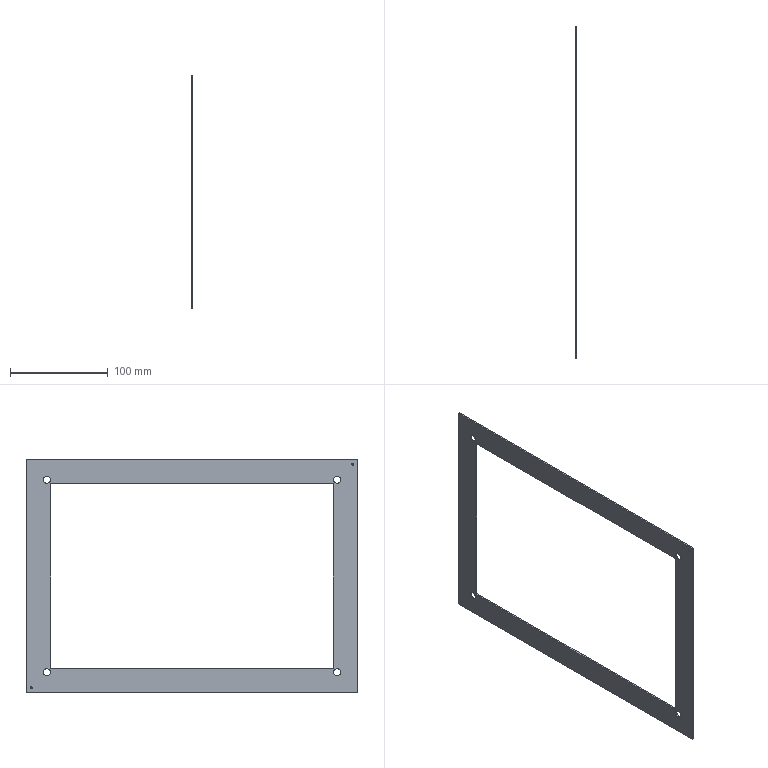Part | SolidWorks | features Extrusion 1 | 1 solid | 22 faces | box 1.5 x 338.6 x 238.5 mm | volume 39286 mm3 | cylinder 12 | plane 10 | commonest cylinder face diameters 7.1 x8 2 x4
STEP:
#1=CARTESIAN_POINT('',(2614.43,1359.3,292.695));
#2=VERTEX_POINT('',#1);
#3=CARTESIAN_POINT('',(2614.43,1359.3,285.595));
#4=VERTEX_POINT('',#3);
#5=CARTESIAN_POINT('',(2614.43,1359.3,289.145));
#6=DIRECTION('',(1.,0.,0.));
#7=DIRECTION('',(0.,0.,1.));
#8=AXIS2_PLACEMENT_3D('',#5,#6,#7);
#9=CIRCLE('',#8,3.55);
#10=EDGE_CURVE('',#2,#4,#9,.T.);
#11=ORIENTED_EDGE('',*,*,#10,.F.);
#12=CARTESIAN_POINT('',(2615.93,1359.3,292.695));
#13=VERTEX_POINT('',#12);
#14=CARTESIAN_POINT('',(2614.43,1359.3,292.695));
#15=DIRECTION('',(1.,0.,0.));
#16=VECTOR('',#15,1000.);
#17=LINE('',#14,#16);
#18=EDGE_CURVE('',#2,#13,#17,.T.);
#19=ORIENTED_EDGE('',*,*,#18,.T.);
#20=CARTESIAN_POINT('',(2615.93,1359.3,285.595));
#21=VERTEX_POINT('',#20);
#22=CARTESIAN_POINT('',(2615.93,1359.3,289.145));
#23=DIRECTION('',(1.,0.,0.));
#24=DIRECTION('',(0.,0.,1.));
#25=AXIS2_PLACEMENT_3D('',#22,#23,#24);
#26=CIRCLE('',#25,3.55);
#27=EDGE_CURVE('',#13,#21,#26,.T.);
#28=ORIENTED_EDGE('',*,*,#27,.T.);
#29=CARTESIAN_POINT('',(2614.43,1359.3,285.595));
#30=DIRECTION('',(1.,0.,0.));
#31=VECTOR('',#30,1000.);
#32=LINE('',#29,#31);
#33=EDGE_CURVE('',#4,#21,#32,.T.);
#34=ORIENTED_EDGE('',*,*,#33,.F.);
#35=EDGE_LOOP('',(#11,#19,#28,#34));
#36=FACE_OUTER_BOUND('',#35,.T.);
#37=CARTESIAN_POINT('',(2614.43,1359.3,289.145));
#38=DIRECTION('',(1.,0.,0.));
#39=DIRECTION('',(0.,0.,-1.));
#40=AXIS2_PLACEMENT_3D('',#37,#38,#39);
#41=CYLINDRICAL_SURFACE('',#40,3.55);
#42=ADVANCED_FACE('',(#36),#41,.F.);
#43=CARTESIAN_POINT('',(2614.43,1062.7,96.195));
#44=VERTEX_POINT('',#43);
#45=CARTESIAN_POINT('',(2614.43,1062.7,89.095));
#46=VERTEX_POINT('',#45);
#47=CARTESIAN_POINT('',(2614.43,1062.7,92.645));
#48=DIRECTION('',(1.,0.,0.));
#49=DIRECTION('',(0.,0.,1.));
#50=AXIS2_PLACEMENT_3D('',#47,#48,#49);
#51=CIRCLE('',#50,3.55);
#52=EDGE_CURVE('',#44,#46,#51,.T.);
#53=ORIENTED_EDGE('',*,*,#52,.F.);
#54=CARTESIAN_POINT('',(2615.93,1062.7,96.195));
#55=VERTEX_POINT('',#54);
#56=CARTESIAN_POINT('',(2614.43,1062.7,96.195));
#57=DIRECTION('',(1.,0.,0.));
#58=VECTOR('',#57,1000.);
#59=LINE('',#56,#58);
#60=EDGE_CURVE('',#44,#55,#59,.T.);
#61=ORIENTED_EDGE('',*,*,#60,.T.);
#62=CARTESIAN_POINT('',(2615.93,1062.7,89.095));
#63=VERTEX_POINT('',#62);
#64=CARTESIAN_POINT('',(2615.93,1062.7,92.645));
#65=DIRECTION('',(1.,0.,0.));
#66=DIRECTION('',(0.,0.,1.));
#67=AXIS2_PLACEMENT_3D('',#64,#65,#66);
#68=CIRCLE('',#67,3.55);
#69=EDGE_CURVE('',#55,#63,#68,.T.);
#70=ORIENTED_EDGE('',*,*,#69,.T.);
#71=CARTESIAN_POINT('',(2614.43,1062.7,89.095));
#72=DIRECTION('',(1.,0.,0.));
#73=VECTOR('',#72,1000.);
#74=LINE('',#71,#73);
#75=EDGE_CURVE('',#46,#63,#74,.T.);
#76=ORIENTED_EDGE('',*,*,#75,.F.);
#77=EDGE_LOOP('',(#53,#61,#70,#76));
#78=FACE_OUTER_BOUND('',#77,.T.);
#79=CARTESIAN_POINT('',(2614.43,1062.7,92.645));
#80=DIRECTION('',(1.,0.,0.));
#81=DIRECTION('',(0.,0.,-1.));
#82=AXIS2_PLACEMENT_3D('',#79,#80,#81);
#83=CYLINDRICAL_SURFACE('',#82,3.55);
#84=ADVANCED_FACE('',(#78),#83,.F.);
#85=CARTESIAN_POINT('',(2614.43,1359.3,96.195));
#86=VERTEX_POINT('',#85);
#87=CARTESIAN_POINT('',(2614.43,1359.3,89.095));
#88=VERTEX_POINT('',#87);
#89=CARTESIAN_POINT('',(2614.43,1359.3,92.645));
#90=DIRECTION('',(1.,0.,0.));
#91=DIRECTION('',(0.,0.,1.));
#92=AXIS2_PLACEMENT_3D('',#89,#90,#91);
#93=CIRCLE('',#92,3.55);
#94=EDGE_CURVE('',#86,#88,#93,.T.);
#95=ORIENTED_EDGE('',*,*,#94,.F.);
#96=CARTESIAN_POINT('',(2615.93,1359.3,96.195));
#97=VERTEX_POINT('',#96);
#98=CARTESIAN_POINT('',(2614.43,1359.3,96.195));
#99=DIRECTION('',(1.,0.,0.));
#100=VECTOR('',#99,1000.);
#101=LINE('',#98,#100);
#102=EDGE_CURVE('',#86,#97,#101,.T.);
#103=ORIENTED_EDGE('',*,*,#102,.T.);
#104=CARTESIAN_POINT('',(2615.93,1359.3,89.095));
#105=VERTEX_POINT('',#104);
#106=CARTESIAN_POINT('',(2615.93,1359.3,92.645));
#107=DIRECTION('',(1.,0.,0.));
#108=DIRECTION('',(0.,0.,1.));
#109=AXIS2_PLACEMENT_3D('',#106,#107,#108);
#110=CIRCLE('',#109,3.55);
#111=EDGE_CURVE('',#97,#105,#110,.T.);
#112=ORIENTED_EDGE('',*,*,#111,.T.);
#113=CARTESIAN_POINT('',(2614.43,1359.3,89.095));
#114=DIRECTION('',(1.,0.,0.));
#115=VECTOR('',#114,1000.);
#116=LINE('',#113,#115);
#117=EDGE_CURVE('',#88,#105,#116,.T.);
#118=ORIENTED_EDGE('',*,*,#117,.F.);
#119=EDGE_LOOP('',(#95,#103,#112,#118));
#120=FACE_OUTER_BOUND('',#119,.T.);
#121=CARTESIAN_POINT('',(2614.43,1359.3,92.645));
#122=DIRECTION('',(1.,0.,0.));
#123=DIRECTION('',(0.,0.,-1.));
#124=AXIS2_PLACEMENT_3D('',#121,#122,#123);
#125=CYLINDRICAL_SURFACE('',#124,3.55);
#126=ADVANCED_FACE('',(#120),#125,.F.);
#127=CARTESIAN_POINT('',(2614.43,1062.7,292.695));
#128=VERTEX_POINT('',#127);
#129=CARTESIAN_POINT('',(2614.43,1062.7,285.595));
#130=VERTEX_POINT('',#129);
#131=CARTESIAN_POINT('',(2614.43,1062.7,289.145));
#132=DIRECTION('',(1.,0.,0.));
#133=DIRECTION('',(0.,0.,1.));
#134=AXIS2_PLACEMENT_3D('',#131,#132,#133);
#135=CIRCLE('',#134,3.55);
#136=EDGE_CURVE('',#128,#130,#135,.T.);
#137=ORIENTED_EDGE('',*,*,#136,.F.);
#138=CARTESIAN_POINT('',(2615.93,1062.7,292.695));
#139=VERTEX_POINT('',#138);
#140=CARTESIAN_POINT('',(2614.43,1062.7,292.695));
#141=DIRECTION('',(1.,0.,0.));
#142=VECTOR('',#141,1000.);
#143=LINE('',#140,#142);
#144=EDGE_CURVE('',#128,#139,#143,.T.);
#145=ORIENTED_EDGE('',*,*,#144,.T.);
#146=CARTESIAN_POINT('',(2615.93,1062.7,285.595));
#147=VERTEX_POINT('',#146);
#148=CARTESIAN_POINT('',(2615.93,1062.7,289.145));
#149=DIRECTION('',(1.,0.,0.));
#150=DIRECTION('',(0.,0.,1.));
#151=AXIS2_PLACEMENT_3D('',#148,#149,#150);
#152=CIRCLE('',#151,3.55);
#153=EDGE_CURVE('',#139,#147,#152,.T.);
#154=ORIENTED_EDGE('',*,*,#153,.T.);
#155=CARTESIAN_POINT('',(2614.43,1062.7,285.595));
#156=DIRECTION('',(1.,0.,0.));
#157=VECTOR('',#156,1000.);
#158=LINE('',#155,#157);
#159=EDGE_CURVE('',#130,#147,#158,.T.);
#160=ORIENTED_EDGE('',*,*,#159,.F.);
#161=EDGE_LOOP('',(#137,#145,#154,#160));
#162=FACE_OUTER_BOUND('',#161,.T.);
#163=CARTESIAN_POINT('',(2614.43,1062.7,289.145));
#164=DIRECTION('',(1.,0.,0.));
#165=DIRECTION('',(0.,0.,-1.));
#166=AXIS2_PLACEMENT_3D('',#163,#164,#165);
#167=CYLINDRICAL_SURFACE('',#166,3.55);
#168=ADVANCED_FACE('',(#162),#167,.F.);
#169=CARTESIAN_POINT('',(2614.43,1375.3,77.645));
#170=VERTEX_POINT('',#169);
#171=CARTESIAN_POINT('',(2614.43,1375.3,75.645));
#172=VERTEX_POINT('',#171);
#173=CARTESIAN_POINT('',(2614.43,1375.3,76.645));
#174=DIRECTION('',(1.,0.,0.));
#175=DIRECTION('',(0.,0.,1.));
#176=AXIS2_PLACEMENT_3D('',#173,#174,#175);
#177=CIRCLE('',#176,1.);
#178=EDGE_CURVE('',#170,#172,#177,.T.);
#179=ORIENTED_EDGE('',*,*,#178,.F.);
#180=CARTESIAN_POINT('',(2615.93,1375.3,77.645));
#181=VERTEX_POINT('',#180);
#182=CARTESIAN_POINT('',(2614.43,1375.3,77.645));
#183=DIRECTION('',(1.,0.,0.));
#184=VECTOR('',#183,1000.);
#185=LINE('',#182,#184);
#186=EDGE_CURVE('',#170,#181,#185,.T.);
#187=ORIENTED_EDGE('',*,*,#186,.T.);
#188=CARTESIAN_POINT('',(2615.93,1375.3,75.645));
#189=VERTEX_POINT('',#188);
#190=CARTESIAN_POINT('',(2615.93,1375.3,76.645));
#191=DIRECTION('',(1.,0.,0.));
#192=DIRECTION('',(0.,0.,1.));
#193=AXIS2_PLACEMENT_3D('',#190,#191,#192);
#194=CIRCLE('',#193,1.);
#195=EDGE_CURVE('',#181,#189,#194,.T.);
#196=ORIENTED_EDGE('',*,*,#195,.T.);
#197=CARTESIAN_POINT('',(2614.43,1375.3,75.645));
#198=DIRECTION('',(1.,0.,0.));
#199=VECTOR('',#198,1000.);
#200=LINE('',#197,#199);
#201=EDGE_CURVE('',#172,#189,#200,.T.);
#202=ORIENTED_EDGE('',*,*,#201,.F.);
#203=EDGE_LOOP('',(#179,#187,#196,#202));
#204=FACE_OUTER_BOUND('',#203,.T.);
#205=CARTESIAN_POINT('',(2614.43,1375.3,76.645));
#206=DIRECTION('',(1.,0.,0.));
#207=DIRECTION('',(0.,0.,-1.));
#208=AXIS2_PLACEMENT_3D('',#205,#206,#207);
#209=CYLINDRICAL_SURFACE('',#208,1.);
#210=ADVANCED_FACE('',(#204),#209,.F.);
#211=CARTESIAN_POINT('',(2614.43,1046.7,306.145));
#212=VERTEX_POINT('',#211);
#213=CARTESIAN_POINT('',(2614.43,1046.7,304.145));
#214=VERTEX_POINT('',#213);
#215=CARTESIAN_POINT('',(2614.43,1046.7,305.145));
#216=DIRECTION('',(1.,0.,0.));
#217=DIRECTION('',(0.,0.,1.));
#218=AXIS2_PLACEMENT_3D('',#215,#216,#217);
#219=CIRCLE('',#218,1.);
#220=EDGE_CURVE('',#212,#214,#219,.T.);
#221=ORIENTED_EDGE('',*,*,#220,.F.);
#222=CARTESIAN_POINT('',(2615.93,1046.7,306.145));
#223=VERTEX_POINT('',#222);
#224=CARTESIAN_POINT('',(2614.43,1046.7,306.145));
#225=DIRECTION('',(1.,0.,0.));
#226=VECTOR('',#225,1000.);
#227=LINE('',#224,#226);
#228=EDGE_CURVE('',#212,#223,#227,.T.);
#229=ORIENTED_EDGE('',*,*,#228,.T.);
#230=CARTESIAN_POINT('',(2615.93,1046.7,304.145));
#231=VERTEX_POINT('',#230);
#232=CARTESIAN_POINT('',(2615.93,1046.7,305.145));
#233=DIRECTION('',(1.,0.,0.));
#234=DIRECTION('',(0.,0.,1.));
#235=AXIS2_PLACEMENT_3D('',#232,#233,#234);
#236=CIRCLE('',#235,1.);
#237=EDGE_CURVE('',#223,#231,#236,.T.);
#238=ORIENTED_EDGE('',*,*,#237,.T.);
#239=CARTESIAN_POINT('',(2614.43,1046.7,304.145));
#240=DIRECTION('',(1.,0.,0.));
#241=VECTOR('',#240,1000.);
#242=LINE('',#239,#241);
#243=EDGE_CURVE('',#214,#231,#242,.T.);
#244=ORIENTED_EDGE('',*,*,#243,.F.);
#245=EDGE_LOOP('',(#221,#229,#238,#244));
#246=FACE_OUTER_BOUND('',#245,.T.);
#247=CARTESIAN_POINT('',(2614.43,1046.7,305.145));
#248=DIRECTION('',(1.,0.,0.));
#249=DIRECTION('',(0.,0.,-1.));
#250=AXIS2_PLACEMENT_3D('',#247,#248,#249);
#251=CYLINDRICAL_SURFACE('',#250,1.);
#252=ADVANCED_FACE('',(#246),#251,.F.);
#253=CARTESIAN_POINT('',(2615.93,1380.3,310.145));
#254=VERTEX_POINT('',#253);
#255=CARTESIAN_POINT('',(2615.93,1041.7,310.145));
#256=VERTEX_POINT('',#255);
#257=CARTESIAN_POINT('',(2615.93,1380.3,310.145));
#258=DIRECTION('',(0.,-1.,0.));
#259=VECTOR('',#258,1000.);
#260=LINE('',#257,#259);
#261=EDGE_CURVE('',#254,#256,#260,.T.);
#262=ORIENTED_EDGE('',*,*,#261,.F.);
#263=CARTESIAN_POINT('',(2614.43,1380.3,310.145));
#264=VERTEX_POINT('',#263);
#265=CARTESIAN_POINT('',(2614.43,1380.3,310.145));
#266=DIRECTION('',(1.,0.,0.));
#267=VECTOR('',#266,1000.);
#268=LINE('',#265,#267);
#269=EDGE_CURVE('',#264,#254,#268,.T.);
#270=ORIENTED_EDGE('',*,*,#269,.F.);
#271=CARTESIAN_POINT('',(2614.43,1041.7,310.145));
#272=VERTEX_POINT('',#271);
#273=CARTESIAN_POINT('',(2614.43,1380.3,310.145));
#274=DIRECTION('',(0.,-1.,0.));
#275=VECTOR('',#274,1000.);
#276=LINE('',#273,#275);
#277=EDGE_CURVE('',#264,#272,#276,.T.);
#278=ORIENTED_EDGE('',*,*,#277,.T.);
#279=CARTESIAN_POINT('',(2614.43,1041.7,310.145));
#280=DIRECTION('',(1.,0.,0.));
#281=VECTOR('',#280,1000.);
#282=LINE('',#279,#281);
#283=EDGE_CURVE('',#272,#256,#282,.T.);
#284=ORIENTED_EDGE('',*,*,#283,.T.);
#285=EDGE_LOOP('',(#262,#270,#278,#284));
#286=FACE_OUTER_BOUND('',#285,.T.);
#287=CARTESIAN_POINT('',(2614.43,1380.3,310.145));
#288=DIRECTION('',(0.,0.,1.));
#289=DIRECTION('',(0.,-1.,0.));
#290=AXIS2_PLACEMENT_3D('',#287,#288,#289);
#291=PLANE('',#290);
#292=ADVANCED_FACE('',(#286),#291,.T.);
#293=CARTESIAN_POINT('',(2615.93,1380.3,71.645));
#294=VERTEX_POINT('',#293);
#295=CARTESIAN_POINT('',(2615.93,1380.3,71.645));
#296=DIRECTION('',(0.,0.,1.));
#297=VECTOR('',#296,1000.);
#298=LINE('',#295,#297);
#299=EDGE_CURVE('',#294,#254,#298,.T.);
#300=ORIENTED_EDGE('',*,*,#299,.F.);
#301=CARTESIAN_POINT('',(2614.43,1380.3,71.645));
#302=VERTEX_POINT('',#301);
#303=CARTESIAN_POINT('',(2614.43,1380.3,71.645));
#304=DIRECTION('',(1.,0.,0.));
#305=VECTOR('',#304,1000.);
#306=LINE('',#303,#305);
#307=EDGE_CURVE('',#302,#294,#306,.T.);
#308=ORIENTED_EDGE('',*,*,#307,.F.);
#309=CARTESIAN_POINT('',(2614.43,1380.3,71.645));
#310=DIRECTION('',(0.,0.,1.));
#311=VECTOR('',#310,1000.);
#312=LINE('',#309,#311);
#313=EDGE_CURVE('',#302,#264,#312,.T.);
#314=ORIENTED_EDGE('',*,*,#313,.T.);
#315=ORIENTED_EDGE('',*,*,#269,.T.);
#316=EDGE_LOOP('',(#300,#308,#314,#315));
#317=FACE_OUTER_BOUND('',#316,.T.);
#318=CARTESIAN_POINT('',(2614.43,1380.3,71.645));
#319=DIRECTION('',(0.,1.,0.));
#320=DIRECTION('',(0.,0.,1.));
#321=AXIS2_PLACEMENT_3D('',#318,#319,#320);
#322=PLANE('',#321);
#323=ADVANCED_FACE('',(#317),#322,.T.);
#324=CARTESIAN_POINT('',(2615.93,1041.7,71.645));
#325=VERTEX_POINT('',#324);
#326=CARTESIAN_POINT('',(2615.93,1041.7,71.645));
#327=DIRECTION('',(0.,1.,0.));
#328=VECTOR('',#327,1000.);
#329=LINE('',#326,#328);
#330=EDGE_CURVE('',#325,#294,#329,.T.);
#331=ORIENTED_EDGE('',*,*,#330,.F.);
#332=CARTESIAN_POINT('',(2614.43,1041.7,71.645));
#333=VERTEX_POINT('',#332);
#334=CARTESIAN_POINT('',(2614.43,1041.7,71.645));
#335=DIRECTION('',(1.,0.,0.));
#336=VECTOR('',#335,1000.);
#337=LINE('',#334,#336);
#338=EDGE_CURVE('',#333,#325,#337,.T.);
#339=ORIENTED_EDGE('',*,*,#338,.F.);
#340=CARTESIAN_POINT('',(2614.43,1041.7,71.645));
#341=DIRECTION('',(0.,1.,0.));
#342=VECTOR('',#341,1000.);
#343=LINE('',#340,#342);
#344=EDGE_CURVE('',#333,#302,#343,.T.);
#345=ORIENTED_EDGE('',*,*,#344,.T.);
#346=ORIENTED_EDGE('',*,*,#307,.T.);
#347=EDGE_LOOP('',(#331,#339,#345,#346));
#348=FACE_OUTER_BOUND('',#347,.T.);
#349=CARTESIAN_POINT('',(2614.43,1041.7,71.645));
#350=DIRECTION('',(0.,0.,-1.));
#351=DIRECTION('',(0.,1.,0.));
#352=AXIS2_PLACEMENT_3D('',#349,#350,#351);
#353=PLANE('',#352);
#354=ADVANCED_FACE('',(#348),#353,.T.);
#355=CARTESIAN_POINT('',(2615.93,1041.7,310.145));
#356=DIRECTION('',(0.,0.,-1.));
#357=VECTOR('',#356,1000.);
#358=LINE('',#355,#357);
#359=EDGE_CURVE('',#256,#325,#358,.T.);
#360=ORIENTED_EDGE('',*,*,#359,.F.);
#361=ORIENTED_EDGE('',*,*,#283,.F.);
#362=CARTESIAN_POINT('',(2614.43,1041.7,310.145));
#363=DIRECTION('',(0.,0.,-1.));
#364=VECTOR('',#363,1000.);
#365=LINE('',#362,#364);
#366=EDGE_CURVE('',#272,#333,#365,.T.);
#367=ORIENTED_EDGE('',*,*,#366,.T.);
#368=ORIENTED_EDGE('',*,*,#338,.T.);
#369=EDGE_LOOP('',(#360,#361,#367,#368));
#370=FACE_OUTER_BOUND('',#369,.T.);
#371=CARTESIAN_POINT('',(2614.43,1041.7,310.145));
#372=DIRECTION('',(0.,-1.,0.));
#373=DIRECTION('',(0.,0.,-1.));
#374=AXIS2_PLACEMENT_3D('',#371,#372,#373);
#375=PLANE('',#374);
#376=ADVANCED_FACE('',(#370),#375,.T.);
#377=CARTESIAN_POINT('',(2614.43,1355.3,285.145));
#378=VERTEX_POINT('',#377);
#379=CARTESIAN_POINT('',(2614.43,1066.7,285.145));
#380=VERTEX_POINT('',#379);
#381=CARTESIAN_POINT('',(2614.43,1066.7,285.145));
#382=DIRECTION('',(0.,-1.,0.));
#383=VECTOR('',#382,1000.);
#384=LINE('',#381,#383);
#385=EDGE_CURVE('',#378,#380,#384,.T.);
#386=ORIENTED_EDGE('',*,*,#385,.T.);
#387=CARTESIAN_POINT('',(2614.43,1066.7,96.645));
#388=VERTEX_POINT('',#387);
#389=CARTESIAN_POINT('',(2614.43,1066.7,96.645));
#390=DIRECTION('',(0.,0.,-1.));
#391=VECTOR('',#390,1000.);
#392=LINE('',#389,#391);
#393=EDGE_CURVE('',#380,#388,#392,.T.);
#394=ORIENTED_EDGE('',*,*,#393,.T.);
#395=CARTESIAN_POINT('',(2614.43,1355.3,96.645));
#396=VERTEX_POINT('',#395);
#397=CARTESIAN_POINT('',(2614.43,1355.3,96.645));
#398=DIRECTION('',(0.,1.,0.));
#399=VECTOR('',#398,1000.);
#400=LINE('',#397,#399);
#401=EDGE_CURVE('',#388,#396,#400,.T.);
#402=ORIENTED_EDGE('',*,*,#401,.T.);
#403=CARTESIAN_POINT('',(2614.43,1355.3,285.145));
#404=DIRECTION('',(0.,0.,1.));
#405=VECTOR('',#404,1000.);
#406=LINE('',#403,#405);
#407=EDGE_CURVE('',#396,#378,#406,.T.);
#408=ORIENTED_EDGE('',*,*,#407,.T.);
#409=EDGE_LOOP('',(#386,#394,#402,#408));
#410=FACE_BOUND('',#409,.T.);
#411=CARTESIAN_POINT('',(2614.43,1359.3,289.145));
#412=DIRECTION('',(1.,0.,0.));
#413=DIRECTION('',(0.,0.,1.));
#414=AXIS2_PLACEMENT_3D('',#411,#412,#413);
#415=CIRCLE('',#414,3.55);
#416=EDGE_CURVE('',#4,#2,#415,.T.);
#417=ORIENTED_EDGE('',*,*,#416,.T.);
#418=ORIENTED_EDGE('',*,*,#10,.T.);
#419=EDGE_LOOP('',(#417,#418));
#420=FACE_BOUND('',#419,.T.);
#421=CARTESIAN_POINT('',(2614.43,1062.7,92.645));
#422=DIRECTION('',(1.,0.,0.));
#423=DIRECTION('',(0.,0.,1.));
#424=AXIS2_PLACEMENT_3D('',#421,#422,#423);
#425=CIRCLE('',#424,3.55);
#426=EDGE_CURVE('',#46,#44,#425,.T.);
#427=ORIENTED_EDGE('',*,*,#426,.T.);
#428=ORIENTED_EDGE('',*,*,#52,.T.);
#429=EDGE_LOOP('',(#427,#428));
#430=FACE_BOUND('',#429,.T.);
#431=CARTESIAN_POINT('',(2614.43,1359.3,92.645));
#432=DIRECTION('',(1.,0.,0.));
#433=DIRECTION('',(0.,0.,1.));
#434=AXIS2_PLACEMENT_3D('',#431,#432,#433);
#435=CIRCLE('',#434,3.55);
#436=EDGE_CURVE('',#88,#86,#435,.T.);
#437=ORIENTED_EDGE('',*,*,#436,.T.);
#438=ORIENTED_EDGE('',*,*,#94,.T.);
#439=EDGE_LOOP('',(#437,#438));
#440=FACE_BOUND('',#439,.T.);
#441=CARTESIAN_POINT('',(2614.43,1062.7,289.145));
#442=DIRECTION('',(1.,0.,0.));
#443=DIRECTION('',(0.,0.,1.));
#444=AXIS2_PLACEMENT_3D('',#441,#442,#443);
#445=CIRCLE('',#444,3.55);
#446=EDGE_CURVE('',#130,#128,#445,.T.);
#447=ORIENTED_EDGE('',*,*,#446,.T.);
#448=ORIENTED_EDGE('',*,*,#136,.T.);
#449=EDGE_LOOP('',(#447,#448));
#450=FACE_BOUND('',#449,.T.);
#451=CARTESIAN_POINT('',(2614.43,1375.3,76.645));
#452=DIRECTION('',(1.,0.,0.));
#453=DIRECTION('',(0.,0.,1.));
#454=AXIS2_PLACEMENT_3D('',#451,#452,#453);
#455=CIRCLE('',#454,1.);
#456=EDGE_CURVE('',#172,#170,#455,.T.);
#457=ORIENTED_EDGE('',*,*,#456,.T.);
#458=ORIENTED_EDGE('',*,*,#178,.T.);
#459=EDGE_LOOP('',(#457,#458));
#460=FACE_BOUND('',#459,.T.);
#461=CARTESIAN_POINT('',(2614.43,1046.7,305.145));
#462=DIRECTION('',(1.,0.,0.));
#463=DIRECTION('',(0.,0.,1.));
#464=AXIS2_PLACEMENT_3D('',#461,#462,#463);
#465=CIRCLE('',#464,1.);
#466=EDGE_CURVE('',#214,#212,#465,.T.);
#467=ORIENTED_EDGE('',*,*,#466,.T.);
#468=ORIENTED_EDGE('',*,*,#220,.T.);
#469=EDGE_LOOP('',(#467,#468));
#470=FACE_BOUND('',#469,.T.);
#471=ORIENTED_EDGE('',*,*,#277,.F.);
#472=ORIENTED_EDGE('',*,*,#313,.F.);
#473=ORIENTED_EDGE('',*,*,#344,.F.);
#474=ORIENTED_EDGE('',*,*,#366,.F.);
#475=EDGE_LOOP('',(#471,#472,#473,#474));
#476=FACE_OUTER_BOUND('',#475,.T.);
#477=CARTESIAN_POINT('',(2614.43,0.,0.));
#478=DIRECTION('',(1.,0.,0.));
#479=DIRECTION('',(0.,0.,-1.));
#480=AXIS2_PLACEMENT_3D('',#477,#478,#479);
#481=PLANE('',#480);
#482=ADVANCED_FACE('',(#410,#420,#430,#440,#450,#460,#470,#476),#481,.F.);
#483=CARTESIAN_POINT('',(2615.93,1066.7,285.145));
#484=VERTEX_POINT('',#483);
#485=CARTESIAN_POINT('',(2615.93,1066.7,96.645));
#486=VERTEX_POINT('',#485);
#487=CARTESIAN_POINT('',(2615.93,1066.7,96.645));
#488=DIRECTION('',(0.,0.,-1.));
#489=VECTOR('',#488,1000.);
#490=LINE('',#487,#489);
#491=EDGE_CURVE('',#484,#486,#490,.T.);
#492=ORIENTED_EDGE('',*,*,#491,.F.);
#493=CARTESIAN_POINT('',(2615.93,1355.3,285.145));
#494=VERTEX_POINT('',#493);
#495=CARTESIAN_POINT('',(2615.93,1066.7,285.145));
#496=DIRECTION('',(0.,-1.,0.));
#497=VECTOR('',#496,1000.);
#498=LINE('',#495,#497);
#499=EDGE_CURVE('',#494,#484,#498,.T.);
#500=ORIENTED_EDGE('',*,*,#499,.F.);
#501=CARTESIAN_POINT('',(2615.93,1355.3,96.645));
#502=VERTEX_POINT('',#501);
#503=CARTESIAN_POINT('',(2615.93,1355.3,285.145));
#504=DIRECTION('',(0.,0.,1.));
#505=VECTOR('',#504,1000.);
#506=LINE('',#503,#505);
#507=EDGE_CURVE('',#502,#494,#506,.T.);
#508=ORIENTED_EDGE('',*,*,#507,.F.);
#509=CARTESIAN_POINT('',(2615.93,1355.3,96.645));
#510=DIRECTION('',(0.,1.,0.));
#511=VECTOR('',#510,1000.);
#512=LINE('',#509,#511);
#513=EDGE_CURVE('',#486,#502,#512,.T.);
#514=ORIENTED_EDGE('',*,*,#513,.F.);
#515=EDGE_LOOP('',(#492,#500,#508,#514));
#516=FACE_BOUND('',#515,.T.);
#517=CARTESIAN_POINT('',(2615.93,1359.3,289.145));
#518=DIRECTION('',(1.,0.,0.));
#519=DIRECTION('',(0.,0.,1.));
#520=AXIS2_PLACEMENT_3D('',#517,#518,#519);
#521=CIRCLE('',#520,3.55);
#522=EDGE_CURVE('',#21,#13,#521,.T.);
#523=ORIENTED_EDGE('',*,*,#522,.F.);
#524=ORIENTED_EDGE('',*,*,#27,.F.);
#525=EDGE_LOOP('',(#523,#524));
#526=FACE_BOUND('',#525,.T.);
#527=CARTESIAN_POINT('',(2615.93,1062.7,92.645));
#528=DIRECTION('',(1.,0.,0.));
#529=DIRECTION('',(0.,0.,1.));
#530=AXIS2_PLACEMENT_3D('',#527,#528,#529);
#531=CIRCLE('',#530,3.55);
#532=EDGE_CURVE('',#63,#55,#531,.T.);
#533=ORIENTED_EDGE('',*,*,#532,.F.);
#534=ORIENTED_EDGE('',*,*,#69,.F.);
#535=EDGE_LOOP('',(#533,#534));
#536=FACE_BOUND('',#535,.T.);
#537=CARTESIAN_POINT('',(2615.93,1359.3,92.645));
#538=DIRECTION('',(1.,0.,0.));
#539=DIRECTION('',(0.,0.,1.));
#540=AXIS2_PLACEMENT_3D('',#537,#538,#539);
#541=CIRCLE('',#540,3.55);
#542=EDGE_CURVE('',#105,#97,#541,.T.);
#543=ORIENTED_EDGE('',*,*,#542,.F.);
#544=ORIENTED_EDGE('',*,*,#111,.F.);
#545=EDGE_LOOP('',(#543,#544));
#546=FACE_BOUND('',#545,.T.);
#547=CARTESIAN_POINT('',(2615.93,1062.7,289.145));
#548=DIRECTION('',(1.,0.,0.));
#549=DIRECTION('',(0.,0.,1.));
#550=AXIS2_PLACEMENT_3D('',#547,#548,#549);
#551=CIRCLE('',#550,3.55);
#552=EDGE_CURVE('',#147,#139,#551,.T.);
#553=ORIENTED_EDGE('',*,*,#552,.F.);
#554=ORIENTED_EDGE('',*,*,#153,.F.);
#555=EDGE_LOOP('',(#553,#554));
#556=FACE_BOUND('',#555,.T.);
#557=CARTESIAN_POINT('',(2615.93,1375.3,76.645));
#558=DIRECTION('',(1.,0.,0.));
#559=DIRECTION('',(0.,0.,1.));
#560=AXIS2_PLACEMENT_3D('',#557,#558,#559);
#561=CIRCLE('',#560,1.);
#562=EDGE_CURVE('',#189,#181,#561,.T.);
#563=ORIENTED_EDGE('',*,*,#562,.F.);
#564=ORIENTED_EDGE('',*,*,#195,.F.);
#565=EDGE_LOOP('',(#563,#564));
#566=FACE_BOUND('',#565,.T.);
#567=CARTESIAN_POINT('',(2615.93,1046.7,305.145));
#568=DIRECTION('',(1.,0.,0.));
#569=DIRECTION('',(0.,0.,1.));
#570=AXIS2_PLACEMENT_3D('',#567,#568,#569);
#571=CIRCLE('',#570,1.);
#572=EDGE_CURVE('',#231,#223,#571,.T.);
#573=ORIENTED_EDGE('',*,*,#572,.F.);
#574=ORIENTED_EDGE('',*,*,#237,.F.);
#575=EDGE_LOOP('',(#573,#574));
#576=FACE_BOUND('',#575,.T.);
#577=ORIENTED_EDGE('',*,*,#261,.T.);
#578=ORIENTED_EDGE('',*,*,#359,.T.);
#579=ORIENTED_EDGE('',*,*,#330,.T.);
#580=ORIENTED_EDGE('',*,*,#299,.T.);
#581=EDGE_LOOP('',(#577,#578,#579,#580));
#582=FACE_OUTER_BOUND('',#581,.T.);
#583=CARTESIAN_POINT('',(2615.93,0.,0.));
#584=DIRECTION('',(1.,0.,0.));
#585=DIRECTION('',(0.,0.,-1.));
#586=AXIS2_PLACEMENT_3D('',#583,#584,#585);
#587=PLANE('',#586);
#588=ADVANCED_FACE('',(#516,#526,#536,#546,#556,#566,#576,#582),#587,.T.);
#589=ORIENTED_EDGE('',*,*,#228,.F.);
#590=ORIENTED_EDGE('',*,*,#466,.F.);
#591=ORIENTED_EDGE('',*,*,#243,.T.);
#592=ORIENTED_EDGE('',*,*,#572,.T.);
#593=EDGE_LOOP('',(#589,#590,#591,#592));
#594=FACE_OUTER_BOUND('',#593,.T.);
#595=CARTESIAN_POINT('',(2614.43,1046.7,305.145));
#596=DIRECTION('',(1.,0.,0.));
#597=DIRECTION('',(0.,0.,-1.));
#598=AXIS2_PLACEMENT_3D('',#595,#596,#597);
#599=CYLINDRICAL_SURFACE('',#598,1.);
#600=ADVANCED_FACE('',(#594),#599,.F.);
#601=ORIENTED_EDGE('',*,*,#186,.F.);
#602=ORIENTED_EDGE('',*,*,#456,.F.);
#603=ORIENTED_EDGE('',*,*,#201,.T.);
#604=ORIENTED_EDGE('',*,*,#562,.T.);
#605=EDGE_LOOP('',(#601,#602,#603,#604));
#606=FACE_OUTER_BOUND('',#605,.T.);
#607=CARTESIAN_POINT('',(2614.43,1375.3,76.645));
#608=DIRECTION('',(1.,0.,0.));
#609=DIRECTION('',(0.,0.,-1.));
#610=AXIS2_PLACEMENT_3D('',#607,#608,#609);
#611=CYLINDRICAL_SURFACE('',#610,1.);
#612=ADVANCED_FACE('',(#606),#611,.F.);
#613=ORIENTED_EDGE('',*,*,#144,.F.);
#614=ORIENTED_EDGE('',*,*,#446,.F.);
#615=ORIENTED_EDGE('',*,*,#159,.T.);
#616=ORIENTED_EDGE('',*,*,#552,.T.);
#617=EDGE_LOOP('',(#613,#614,#615,#616));
#618=FACE_OUTER_BOUND('',#617,.T.);
#619=CARTESIAN_POINT('',(2614.43,1062.7,289.145));
#620=DIRECTION('',(1.,0.,0.));
#621=DIRECTION('',(0.,0.,-1.));
#622=AXIS2_PLACEMENT_3D('',#619,#620,#621);
#623=CYLINDRICAL_SURFACE('',#622,3.55);
#624=ADVANCED_FACE('',(#618),#623,.F.);
#625=ORIENTED_EDGE('',*,*,#102,.F.);
#626=ORIENTED_EDGE('',*,*,#436,.F.);
#627=ORIENTED_EDGE('',*,*,#117,.T.);
#628=ORIENTED_EDGE('',*,*,#542,.T.);
#629=EDGE_LOOP('',(#625,#626,#627,#628));
#630=FACE_OUTER_BOUND('',#629,.T.);
#631=CARTESIAN_POINT('',(2614.43,1359.3,92.645));
#632=DIRECTION('',(1.,0.,0.));
#633=DIRECTION('',(0.,0.,-1.));
#634=AXIS2_PLACEMENT_3D('',#631,#632,#633);
#635=CYLINDRICAL_SURFACE('',#634,3.55);
#636=ADVANCED_FACE('',(#630),#635,.F.);
#637=ORIENTED_EDGE('',*,*,#60,.F.);
#638=ORIENTED_EDGE('',*,*,#426,.F.);
#639=ORIENTED_EDGE('',*,*,#75,.T.);
#640=ORIENTED_EDGE('',*,*,#532,.T.);
#641=EDGE_LOOP('',(#637,#638,#639,#640));
#642=FACE_OUTER_BOUND('',#641,.T.);
#643=CARTESIAN_POINT('',(2614.43,1062.7,92.645));
#644=DIRECTION('',(1.,0.,0.));
#645=DIRECTION('',(0.,0.,-1.));
#646=AXIS2_PLACEMENT_3D('',#643,#644,#645);
#647=CYLINDRICAL_SURFACE('',#646,3.55);
#648=ADVANCED_FACE('',(#642),#647,.F.);
#649=ORIENTED_EDGE('',*,*,#18,.F.);
#650=ORIENTED_EDGE('',*,*,#416,.F.);
#651=ORIENTED_EDGE('',*,*,#33,.T.);
#652=ORIENTED_EDGE('',*,*,#522,.T.);
#653=EDGE_LOOP('',(#649,#650,#651,#652));
#654=FACE_OUTER_BOUND('',#653,.T.);
#655=CARTESIAN_POINT('',(2614.43,1359.3,289.145));
#656=DIRECTION('',(1.,0.,0.));
#657=DIRECTION('',(0.,0.,-1.));
#658=AXIS2_PLACEMENT_3D('',#655,#656,#657);
#659=CYLINDRICAL_SURFACE('',#658,3.55);
#660=ADVANCED_FACE('',(#654),#659,.F.);
#661=ORIENTED_EDGE('',*,*,#491,.T.);
#662=CARTESIAN_POINT('',(2614.43,1066.7,96.645));
#663=DIRECTION('',(1.,0.,0.));
#664=VECTOR('',#663,1000.);
#665=LINE('',#662,#664);
#666=EDGE_CURVE('',#388,#486,#665,.T.);
#667=ORIENTED_EDGE('',*,*,#666,.F.);
#668=ORIENTED_EDGE('',*,*,#393,.F.);
#669=CARTESIAN_POINT('',(2614.43,1066.7,285.145));
#670=DIRECTION('',(1.,0.,0.));
#671=VECTOR('',#670,1000.);
#672=LINE('',#669,#671);
#673=EDGE_CURVE('',#380,#484,#672,.T.);
#674=ORIENTED_EDGE('',*,*,#673,.T.);
#675=EDGE_LOOP('',(#661,#667,#668,#674));
#676=FACE_OUTER_BOUND('',#675,.T.);
#677=CARTESIAN_POINT('',(2614.43,1066.7,96.645));
#678=DIRECTION('',(0.,-1.,0.));
#679=DIRECTION('',(0.,0.,-1.));
#680=AXIS2_PLACEMENT_3D('',#677,#678,#679);
#681=PLANE('',#680);
#682=ADVANCED_FACE('',(#676),#681,.F.);
#683=ORIENTED_EDGE('',*,*,#499,.T.);
#684=ORIENTED_EDGE('',*,*,#673,.F.);
#685=ORIENTED_EDGE('',*,*,#385,.F.);
#686=CARTESIAN_POINT('',(2614.43,1355.3,285.145));
#687=DIRECTION('',(1.,0.,0.));
#688=VECTOR('',#687,1000.);
#689=LINE('',#686,#688);
#690=EDGE_CURVE('',#378,#494,#689,.T.);
#691=ORIENTED_EDGE('',*,*,#690,.T.);
#692=EDGE_LOOP('',(#683,#684,#685,#691));
#693=FACE_OUTER_BOUND('',#692,.T.);
#694=CARTESIAN_POINT('',(2614.43,1066.7,285.145));
#695=DIRECTION('',(0.,0.,1.));
#696=DIRECTION('',(1.,0.,0.));
#697=AXIS2_PLACEMENT_3D('',#694,#695,#696);
#698=PLANE('',#697);
#699=ADVANCED_FACE('',(#693),#698,.F.);
#700=ORIENTED_EDGE('',*,*,#507,.T.);
#701=ORIENTED_EDGE('',*,*,#690,.F.);
#702=ORIENTED_EDGE('',*,*,#407,.F.);
#703=CARTESIAN_POINT('',(2614.43,1355.3,96.645));
#704=DIRECTION('',(1.,0.,0.));
#705=VECTOR('',#704,1000.);
#706=LINE('',#703,#705);
#707=EDGE_CURVE('',#396,#502,#706,.T.);
#708=ORIENTED_EDGE('',*,*,#707,.T.);
#709=EDGE_LOOP('',(#700,#701,#702,#708));
#710=FACE_OUTER_BOUND('',#709,.T.);
#711=CARTESIAN_POINT('',(2614.43,1355.3,285.145));
#712=DIRECTION('',(0.,1.,0.));
#713=DIRECTION('',(0.,0.,1.));
#714=AXIS2_PLACEMENT_3D('',#711,#712,#713);
#715=PLANE('',#714);
#716=ADVANCED_FACE('',(#710),#715,.F.);
#717=ORIENTED_EDGE('',*,*,#513,.T.);
#718=ORIENTED_EDGE('',*,*,#707,.F.);
#719=ORIENTED_EDGE('',*,*,#401,.F.);
#720=ORIENTED_EDGE('',*,*,#666,.T.);
#721=EDGE_LOOP('',(#717,#718,#719,#720));
#722=FACE_OUTER_BOUND('',#721,.T.);
#723=CARTESIAN_POINT('',(2614.43,1355.3,96.645));
#724=DIRECTION('',(0.,0.,-1.));
#725=DIRECTION('',(0.,1.,0.));
#726=AXIS2_PLACEMENT_3D('',#723,#724,#725);
#727=PLANE('',#726);
#728=ADVANCED_FACE('',(#722),#727,.F.);
#729=CLOSED_SHELL('',(#42,#84,#126,#168,#210,#252,#292,#323,#354,#376,#482,#588,#600,#612,#624,#636,#648,#660,#682,#699,#716,#728));
#730=MANIFOLD_SOLID_BREP('',#729);
#731=CARTESIAN_POINT('',(0.,0.,0.));
#732=DIRECTION('',(0.,0.,1.));
#733=DIRECTION('',(1.,0.,0.));
#734=AXIS2_PLACEMENT_3D('',#731,#732,#733);
#735=(LENGTH_UNIT()NAMED_UNIT(*)SI_UNIT(.MILLI.,.METRE.));
#736=UNCERTAINTY_MEASURE_WITH_UNIT(LENGTH_MEASURE(0.00001),#735,'','');
#737=(NAMED_UNIT(*)PLANE_ANGLE_UNIT()SI_UNIT($,.RADIAN.));
#738=(NAMED_UNIT(*)SI_UNIT($,.STERADIAN.)SOLID_ANGLE_UNIT());
#739=(GEOMETRIC_REPRESENTATION_CONTEXT(3)GLOBAL_UNCERTAINTY_ASSIGNED_CONTEXT((#736))GLOBAL_UNIT_ASSIGNED_CONTEXT((#735,#737,#738))REPRESENTATION_CONTEXT('',''));
#740=ADVANCED_BREP_SHAPE_REPRESENTATION('',(#730,#734),#739);